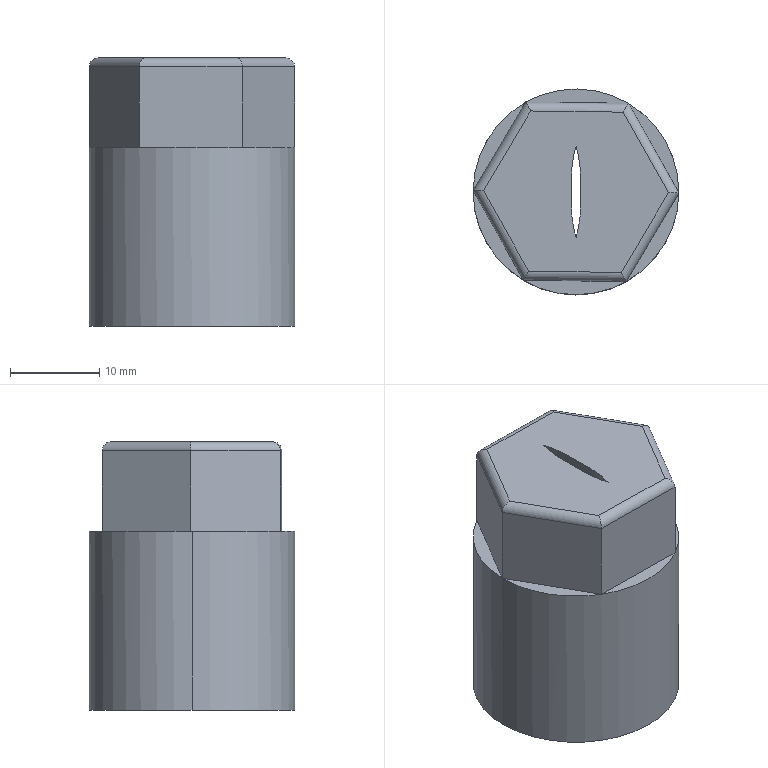Part | SolidWorks | features ICE 3, Extrusion 1, Fillet 1 | 1 solid | 35 faces | box 23 x 23 x 30 mm | volume 5402 mm3 | plane 21 | cylinder 14 | commonest cylinder face diameters 2 x6 20 x4 21 x2 23 x2
STEP:
#1=CARTESIAN_POINT('',(10.5,0.,18.));
#2=VERTEX_POINT('',#1);
#3=CARTESIAN_POINT('',(-10.5,0.,18.));
#4=VERTEX_POINT('',#3);
#5=CARTESIAN_POINT('',(0.,0.,18.));
#6=DIRECTION('',(0.,0.,-1.));
#7=DIRECTION('',(-1.,0.,0.));
#8=AXIS2_PLACEMENT_3D('',#5,#6,#7);
#9=CIRCLE('',#8,10.5);
#10=EDGE_CURVE('',#2,#4,#9,.T.);
#11=ORIENTED_EDGE('',*,*,#10,.F.);
#12=CARTESIAN_POINT('',(10.5,0.,0.));
#13=VERTEX_POINT('',#12);
#14=CARTESIAN_POINT('',(10.5,0.,18.));
#15=DIRECTION('',(0.,0.,-1.));
#16=VECTOR('',#15,1000.);
#17=LINE('',#14,#16);
#18=EDGE_CURVE('',#2,#13,#17,.T.);
#19=ORIENTED_EDGE('',*,*,#18,.T.);
#20=CARTESIAN_POINT('',(-10.5,0.,0.));
#21=VERTEX_POINT('',#20);
#22=CARTESIAN_POINT('',(0.,0.,0.));
#23=DIRECTION('',(0.,0.,-1.));
#24=DIRECTION('',(-1.,0.,0.));
#25=AXIS2_PLACEMENT_3D('',#22,#23,#24);
#26=CIRCLE('',#25,10.5);
#27=EDGE_CURVE('',#13,#21,#26,.T.);
#28=ORIENTED_EDGE('',*,*,#27,.T.);
#29=CARTESIAN_POINT('',(-10.5,0.,18.));
#30=DIRECTION('',(0.,0.,-1.));
#31=VECTOR('',#30,1000.);
#32=LINE('',#29,#31);
#33=EDGE_CURVE('',#4,#21,#32,.T.);
#34=ORIENTED_EDGE('',*,*,#33,.F.);
#35=EDGE_LOOP('',(#11,#19,#28,#34));
#36=FACE_OUTER_BOUND('',#35,.T.);
#37=CARTESIAN_POINT('',(0.,0.,18.));
#38=DIRECTION('',(0.,0.,-1.));
#39=DIRECTION('',(-1.,0.,0.));
#40=AXIS2_PLACEMENT_3D('',#37,#38,#39);
#41=CYLINDRICAL_SURFACE('',#40,10.5);
#42=ADVANCED_FACE('',(#36),#41,.F.);
#43=CARTESIAN_POINT('',(11.5,0.,20.));
#44=VERTEX_POINT('',#43);
#45=CARTESIAN_POINT('',(5.876,9.886,20.));
#46=VERTEX_POINT('',#45);
#47=CARTESIAN_POINT('',(0.,0.,20.));
#48=DIRECTION('',(0.,0.,1.));
#49=DIRECTION('',(1.,0.,0.));
#50=AXIS2_PLACEMENT_3D('',#47,#48,#49);
#51=CIRCLE('',#50,11.5);
#52=EDGE_CURVE('',#44,#46,#51,.T.);
#53=ORIENTED_EDGE('',*,*,#52,.F.);
#54=CARTESIAN_POINT('',(11.5,0.,0.));
#55=VERTEX_POINT('',#54);
#56=CARTESIAN_POINT('',(11.5,0.,30.));
#57=DIRECTION('',(0.,0.,-1.));
#58=VECTOR('',#57,1000.);
#59=LINE('',#56,#58);
#60=EDGE_CURVE('',#44,#55,#59,.T.);
#61=ORIENTED_EDGE('',*,*,#60,.T.);
#62=CARTESIAN_POINT('',(-11.5,0.,0.));
#63=VERTEX_POINT('',#62);
#64=CARTESIAN_POINT('',(0.,0.,0.));
#65=DIRECTION('',(0.,0.,1.));
#66=DIRECTION('',(1.,0.,0.));
#67=AXIS2_PLACEMENT_3D('',#64,#65,#66);
#68=CIRCLE('',#67,11.5);
#69=EDGE_CURVE('',#55,#63,#68,.T.);
#70=ORIENTED_EDGE('',*,*,#69,.T.);
#71=CARTESIAN_POINT('',(-11.5,0.,20.));
#72=VERTEX_POINT('',#71);
#73=CARTESIAN_POINT('',(-11.5,0.,30.));
#74=DIRECTION('',(0.,0.,-1.));
#75=VECTOR('',#74,1000.);
#76=LINE('',#73,#75);
#77=EDGE_CURVE('',#72,#63,#76,.T.);
#78=ORIENTED_EDGE('',*,*,#77,.F.);
#79=CARTESIAN_POINT('',(-11.499,0.1458,20.));
#80=VERTEX_POINT('',#79);
#81=CARTESIAN_POINT('',(0.,0.,20.));
#82=DIRECTION('',(0.,0.,1.));
#83=DIRECTION('',(1.,0.,0.));
#84=AXIS2_PLACEMENT_3D('',#81,#82,#83);
#85=CIRCLE('',#84,11.5);
#86=EDGE_CURVE('',#80,#72,#85,.T.);
#87=ORIENTED_EDGE('',*,*,#86,.F.);
#88=CARTESIAN_POINT('',(-5.623,10.031,20.));
#89=VERTEX_POINT('',#88);
#90=CARTESIAN_POINT('',(0.,0.,20.));
#91=DIRECTION('',(0.,0.,1.));
#92=DIRECTION('',(1.,0.,0.));
#93=AXIS2_PLACEMENT_3D('',#90,#91,#92);
#94=CIRCLE('',#93,11.5);
#95=EDGE_CURVE('',#89,#80,#94,.T.);
#96=ORIENTED_EDGE('',*,*,#95,.F.);
#97=CARTESIAN_POINT('',(0.,0.,20.));
#98=DIRECTION('',(0.,0.,1.));
#99=DIRECTION('',(1.,0.,0.));
#100=AXIS2_PLACEMENT_3D('',#97,#98,#99);
#101=CIRCLE('',#100,11.5);
#102=EDGE_CURVE('',#46,#89,#101,.T.);
#103=ORIENTED_EDGE('',*,*,#102,.F.);
#104=EDGE_LOOP('',(#53,#61,#70,#78,#87,#96,#103));
#105=FACE_OUTER_BOUND('',#104,.T.);
#106=CARTESIAN_POINT('',(0.,0.,30.));
#107=DIRECTION('',(0.,0.,-1.));
#108=DIRECTION('',(-1.,0.,0.));
#109=AXIS2_PLACEMENT_3D('',#106,#107,#108);
#110=CYLINDRICAL_SURFACE('',#109,11.5);
#111=ADVANCED_FACE('',(#105),#110,.T.);
#112=CARTESIAN_POINT('',(-0.2252,4.148,18.));
#113=VERTEX_POINT('',#112);
#114=CARTESIAN_POINT('',(-0.5,1.82,18.));
#115=VERTEX_POINT('',#114);
#116=CARTESIAN_POINT('',(9.5,1.82,18.));
#117=DIRECTION('',(0.,0.,1.));
#118=DIRECTION('',(-1.,0.,0.));
#119=AXIS2_PLACEMENT_3D('',#116,#117,#118);
#120=CIRCLE('',#119,10.);
#121=EDGE_CURVE('',#113,#115,#120,.T.);
#122=ORIENTED_EDGE('',*,*,#121,.F.);
#123=CARTESIAN_POINT('',(-0.2252,4.148,30.));
#124=VERTEX_POINT('',#123);
#125=CARTESIAN_POINT('',(-0.2252,4.148,0.));
#126=DIRECTION('',(0.,0.,1.));
#127=VECTOR('',#126,1000.);
#128=LINE('',#125,#127);
#129=EDGE_CURVE('',#113,#124,#128,.T.);
#130=ORIENTED_EDGE('',*,*,#129,.T.);
#131=CARTESIAN_POINT('',(-0.5,1.82,30.));
#132=VERTEX_POINT('',#131);
#133=CARTESIAN_POINT('',(9.5,1.82,30.));
#134=DIRECTION('',(0.,0.,1.));
#135=DIRECTION('',(-1.,0.,0.));
#136=AXIS2_PLACEMENT_3D('',#133,#134,#135);
#137=CIRCLE('',#136,10.);
#138=EDGE_CURVE('',#124,#132,#137,.T.);
#139=ORIENTED_EDGE('',*,*,#138,.T.);
#140=CARTESIAN_POINT('',(-0.5,1.82,0.));
#141=DIRECTION('',(0.,0.,1.));
#142=VECTOR('',#141,1000.);
#143=LINE('',#140,#142);
#144=EDGE_CURVE('',#115,#132,#143,.T.);
#145=ORIENTED_EDGE('',*,*,#144,.F.);
#146=EDGE_LOOP('',(#122,#130,#139,#145));
#147=FACE_OUTER_BOUND('',#146,.T.);
#148=CARTESIAN_POINT('',(9.5,1.82,0.));
#149=DIRECTION('',(0.,0.,1.));
#150=DIRECTION('',(1.,0.,0.));
#151=AXIS2_PLACEMENT_3D('',#148,#149,#150);
#152=CYLINDRICAL_SURFACE('',#151,10.);
#153=ADVANCED_FACE('',(#147),#152,.F.);
#154=CARTESIAN_POINT('',(0.,5.089,18.));
#155=VERTEX_POINT('',#154);
#156=CARTESIAN_POINT('',(-0.2252,4.148,18.));
#157=DIRECTION('',(-0.2328,-0.9725,0.));
#158=VECTOR('',#157,1000.);
#159=LINE('',#156,#158);
#160=EDGE_CURVE('',#155,#113,#159,.T.);
#161=ORIENTED_EDGE('',*,*,#160,.F.);
#162=CARTESIAN_POINT('',(0.,5.089,30.));
#163=VERTEX_POINT('',#162);
#164=CARTESIAN_POINT('',(0.,5.089,0.));
#165=DIRECTION('',(0.,0.,1.));
#166=VECTOR('',#165,1000.);
#167=LINE('',#164,#166);
#168=EDGE_CURVE('',#155,#163,#167,.T.);
#169=ORIENTED_EDGE('',*,*,#168,.T.);
#170=CARTESIAN_POINT('',(-0.2252,4.148,30.));
#171=DIRECTION('',(-0.2328,-0.9725,0.));
#172=VECTOR('',#171,1000.);
#173=LINE('',#170,#172);
#174=EDGE_CURVE('',#163,#124,#173,.T.);
#175=ORIENTED_EDGE('',*,*,#174,.T.);
#176=ORIENTED_EDGE('',*,*,#129,.F.);
#177=EDGE_LOOP('',(#161,#169,#175,#176));
#178=FACE_OUTER_BOUND('',#177,.T.);
#179=CARTESIAN_POINT('',(-0.2252,4.148,0.));
#180=DIRECTION('',(-0.9725,0.2328,0.));
#181=DIRECTION('',(-0.2328,-0.9725,0.));
#182=AXIS2_PLACEMENT_3D('',#179,#180,#181);
#183=PLANE('',#182);
#184=ADVANCED_FACE('',(#178),#183,.F.);
#185=CARTESIAN_POINT('',(0.2252,4.148,18.));
#186=VERTEX_POINT('',#185);
#187=CARTESIAN_POINT('',(0.,5.089,18.));
#188=DIRECTION('',(-0.2328,0.9725,0.));
#189=VECTOR('',#188,1000.);
#190=LINE('',#187,#189);
#191=EDGE_CURVE('',#186,#155,#190,.T.);
#192=ORIENTED_EDGE('',*,*,#191,.F.);
#193=CARTESIAN_POINT('',(0.2252,4.148,30.));
#194=VERTEX_POINT('',#193);
#195=CARTESIAN_POINT('',(0.2252,4.148,0.));
#196=DIRECTION('',(0.,0.,1.));
#197=VECTOR('',#196,1000.);
#198=LINE('',#195,#197);
#199=EDGE_CURVE('',#186,#194,#198,.T.);
#200=ORIENTED_EDGE('',*,*,#199,.T.);
#201=CARTESIAN_POINT('',(0.,5.089,30.));
#202=DIRECTION('',(-0.2328,0.9725,0.));
#203=VECTOR('',#202,1000.);
#204=LINE('',#201,#203);
#205=EDGE_CURVE('',#194,#163,#204,.T.);
#206=ORIENTED_EDGE('',*,*,#205,.T.);
#207=ORIENTED_EDGE('',*,*,#168,.F.);
#208=EDGE_LOOP('',(#192,#200,#206,#207));
#209=FACE_OUTER_BOUND('',#208,.T.);
#210=CARTESIAN_POINT('',(0.,5.089,0.));
#211=DIRECTION('',(0.9725,0.2328,0.));
#212=DIRECTION('',(-0.2328,0.9725,0.));
#213=AXIS2_PLACEMENT_3D('',#210,#211,#212);
#214=PLANE('',#213);
#215=ADVANCED_FACE('',(#209),#214,.F.);
#216=CARTESIAN_POINT('',(0.5,1.82,18.));
#217=VERTEX_POINT('',#216);
#218=CARTESIAN_POINT('',(-9.5,1.82,18.));
#219=DIRECTION('',(0.,0.,1.));
#220=DIRECTION('',(-1.,0.,0.));
#221=AXIS2_PLACEMENT_3D('',#218,#219,#220);
#222=CIRCLE('',#221,10.);
#223=EDGE_CURVE('',#217,#186,#222,.T.);
#224=ORIENTED_EDGE('',*,*,#223,.F.);
#225=CARTESIAN_POINT('',(0.5,1.82,30.));
#226=VERTEX_POINT('',#225);
#227=CARTESIAN_POINT('',(0.5,1.82,0.));
#228=DIRECTION('',(0.,0.,1.));
#229=VECTOR('',#228,1000.);
#230=LINE('',#227,#229);
#231=EDGE_CURVE('',#217,#226,#230,.T.);
#232=ORIENTED_EDGE('',*,*,#231,.T.);
#233=CARTESIAN_POINT('',(-9.5,1.82,30.));
#234=DIRECTION('',(0.,0.,1.));
#235=DIRECTION('',(1.,0.,0.));
#236=AXIS2_PLACEMENT_3D('',#233,#234,#235);
#237=CIRCLE('',#236,10.);
#238=EDGE_CURVE('',#226,#194,#237,.T.);
#239=ORIENTED_EDGE('',*,*,#238,.T.);
#240=ORIENTED_EDGE('',*,*,#199,.F.);
#241=EDGE_LOOP('',(#224,#232,#239,#240));
#242=FACE_OUTER_BOUND('',#241,.T.);
#243=CARTESIAN_POINT('',(-9.5,1.82,0.));
#244=DIRECTION('',(0.,0.,1.));
#245=DIRECTION('',(1.,0.,0.));
#246=AXIS2_PLACEMENT_3D('',#243,#244,#245);
#247=CYLINDRICAL_SURFACE('',#246,10.);
#248=ADVANCED_FACE('',(#242),#247,.F.);
#249=CARTESIAN_POINT('',(0.5,-1.82,18.));
#250=VERTEX_POINT('',#249);
#251=CARTESIAN_POINT('',(0.5,0.,18.));
#252=DIRECTION('',(0.,1.,0.));
#253=VECTOR('',#252,1000.);
#254=LINE('',#251,#253);
#255=EDGE_CURVE('',#250,#217,#254,.T.);
#256=ORIENTED_EDGE('',*,*,#255,.F.);
#257=CARTESIAN_POINT('',(0.5,-1.82,30.));
#258=VERTEX_POINT('',#257);
#259=CARTESIAN_POINT('',(0.5,-1.82,0.));
#260=DIRECTION('',(0.,0.,1.));
#261=VECTOR('',#260,1000.);
#262=LINE('',#259,#261);
#263=EDGE_CURVE('',#250,#258,#262,.T.);
#264=ORIENTED_EDGE('',*,*,#263,.T.);
#265=CARTESIAN_POINT('',(0.5,0.,30.));
#266=DIRECTION('',(0.,1.,0.));
#267=VECTOR('',#266,1000.);
#268=LINE('',#265,#267);
#269=EDGE_CURVE('',#258,#226,#268,.T.);
#270=ORIENTED_EDGE('',*,*,#269,.T.);
#271=ORIENTED_EDGE('',*,*,#231,.F.);
#272=EDGE_LOOP('',(#256,#264,#270,#271));
#273=FACE_OUTER_BOUND('',#272,.T.);
#274=CARTESIAN_POINT('',(0.5,0.,0.));
#275=DIRECTION('',(1.,0.,0.));
#276=DIRECTION('',(0.,0.,-1.));
#277=AXIS2_PLACEMENT_3D('',#274,#275,#276);
#278=PLANE('',#277);
#279=ADVANCED_FACE('',(#273),#278,.F.);
#280=CARTESIAN_POINT('',(0.2252,-4.148,18.));
#281=VERTEX_POINT('',#280);
#282=CARTESIAN_POINT('',(-9.5,-1.82,18.));
#283=DIRECTION('',(0.,0.,1.));
#284=DIRECTION('',(-1.,0.,0.));
#285=AXIS2_PLACEMENT_3D('',#282,#283,#284);
#286=CIRCLE('',#285,10.);
#287=EDGE_CURVE('',#281,#250,#286,.T.);
#288=ORIENTED_EDGE('',*,*,#287,.F.);
#289=CARTESIAN_POINT('',(0.2252,-4.148,30.));
#290=VERTEX_POINT('',#289);
#291=CARTESIAN_POINT('',(0.2252,-4.148,0.));
#292=DIRECTION('',(0.,0.,1.));
#293=VECTOR('',#292,1000.);
#294=LINE('',#291,#293);
#295=EDGE_CURVE('',#281,#290,#294,.T.);
#296=ORIENTED_EDGE('',*,*,#295,.T.);
#297=CARTESIAN_POINT('',(-9.5,-1.82,30.));
#298=DIRECTION('',(0.,0.,1.));
#299=DIRECTION('',(1.,0.,0.));
#300=AXIS2_PLACEMENT_3D('',#297,#298,#299);
#301=CIRCLE('',#300,10.);
#302=EDGE_CURVE('',#290,#258,#301,.T.);
#303=ORIENTED_EDGE('',*,*,#302,.T.);
#304=ORIENTED_EDGE('',*,*,#263,.F.);
#305=EDGE_LOOP('',(#288,#296,#303,#304));
#306=FACE_OUTER_BOUND('',#305,.T.);
#307=CARTESIAN_POINT('',(-9.5,-1.82,0.));
#308=DIRECTION('',(0.,0.,1.));
#309=DIRECTION('',(1.,0.,0.));
#310=AXIS2_PLACEMENT_3D('',#307,#308,#309);
#311=CYLINDRICAL_SURFACE('',#310,10.);
#312=ADVANCED_FACE('',(#306),#311,.F.);
#313=CARTESIAN_POINT('',(0.,-5.089,18.));
#314=VERTEX_POINT('',#313);
#315=CARTESIAN_POINT('',(0.,-5.089,18.));
#316=DIRECTION('',(0.2328,0.9725,0.));
#317=VECTOR('',#316,1000.);
#318=LINE('',#315,#317);
#319=EDGE_CURVE('',#314,#281,#318,.T.);
#320=ORIENTED_EDGE('',*,*,#319,.F.);
#321=CARTESIAN_POINT('',(0.,-5.089,30.));
#322=VERTEX_POINT('',#321);
#323=CARTESIAN_POINT('',(0.,-5.089,0.));
#324=DIRECTION('',(0.,0.,1.));
#325=VECTOR('',#324,1000.);
#326=LINE('',#323,#325);
#327=EDGE_CURVE('',#314,#322,#326,.T.);
#328=ORIENTED_EDGE('',*,*,#327,.T.);
#329=CARTESIAN_POINT('',(0.,-5.089,30.));
#330=DIRECTION('',(0.2328,0.9725,0.));
#331=VECTOR('',#330,1000.);
#332=LINE('',#329,#331);
#333=EDGE_CURVE('',#322,#290,#332,.T.);
#334=ORIENTED_EDGE('',*,*,#333,.T.);
#335=ORIENTED_EDGE('',*,*,#295,.F.);
#336=EDGE_LOOP('',(#320,#328,#334,#335));
#337=FACE_OUTER_BOUND('',#336,.T.);
#338=CARTESIAN_POINT('',(0.,-5.089,0.));
#339=DIRECTION('',(0.9725,-0.2328,0.));
#340=DIRECTION('',(0.2328,0.9725,0.));
#341=AXIS2_PLACEMENT_3D('',#338,#339,#340);
#342=PLANE('',#341);
#343=ADVANCED_FACE('',(#337),#342,.F.);
#344=CARTESIAN_POINT('',(-0.2252,-4.148,18.));
#345=VERTEX_POINT('',#344);
#346=CARTESIAN_POINT('',(-0.2252,-4.148,18.));
#347=DIRECTION('',(0.2328,-0.9725,0.));
#348=VECTOR('',#347,1000.);
#349=LINE('',#346,#348);
#350=EDGE_CURVE('',#345,#314,#349,.T.);
#351=ORIENTED_EDGE('',*,*,#350,.F.);
#352=CARTESIAN_POINT('',(-0.2252,-4.148,30.));
#353=VERTEX_POINT('',#352);
#354=CARTESIAN_POINT('',(-0.2252,-4.148,0.));
#355=DIRECTION('',(0.,0.,1.));
#356=VECTOR('',#355,1000.);
#357=LINE('',#354,#356);
#358=EDGE_CURVE('',#345,#353,#357,.T.);
#359=ORIENTED_EDGE('',*,*,#358,.T.);
#360=CARTESIAN_POINT('',(-0.2252,-4.148,30.));
#361=DIRECTION('',(0.2328,-0.9725,0.));
#362=VECTOR('',#361,1000.);
#363=LINE('',#360,#362);
#364=EDGE_CURVE('',#353,#322,#363,.T.);
#365=ORIENTED_EDGE('',*,*,#364,.T.);
#366=ORIENTED_EDGE('',*,*,#327,.F.);
#367=EDGE_LOOP('',(#351,#359,#365,#366));
#368=FACE_OUTER_BOUND('',#367,.T.);
#369=CARTESIAN_POINT('',(-0.2252,-4.148,0.));
#370=DIRECTION('',(-0.9725,-0.2328,0.));
#371=DIRECTION('',(0.2328,-0.9725,0.));
#372=AXIS2_PLACEMENT_3D('',#369,#370,#371);
#373=PLANE('',#372);
#374=ADVANCED_FACE('',(#368),#373,.F.);
#375=CARTESIAN_POINT('',(-0.5,-1.82,18.));
#376=VERTEX_POINT('',#375);
#377=CARTESIAN_POINT('',(9.5,-1.82,18.));
#378=DIRECTION('',(0.,0.,1.));
#379=DIRECTION('',(-1.,0.,0.));
#380=AXIS2_PLACEMENT_3D('',#377,#378,#379);
#381=CIRCLE('',#380,10.);
#382=EDGE_CURVE('',#376,#345,#381,.T.);
#383=ORIENTED_EDGE('',*,*,#382,.F.);
#384=CARTESIAN_POINT('',(-0.5,-1.82,30.));
#385=VERTEX_POINT('',#384);
#386=CARTESIAN_POINT('',(-0.5,-1.82,0.));
#387=DIRECTION('',(0.,0.,1.));
#388=VECTOR('',#387,1000.);
#389=LINE('',#386,#388);
#390=EDGE_CURVE('',#376,#385,#389,.T.);
#391=ORIENTED_EDGE('',*,*,#390,.T.);
#392=CARTESIAN_POINT('',(9.5,-1.82,30.));
#393=DIRECTION('',(0.,0.,1.));
#394=DIRECTION('',(1.,0.,0.));
#395=AXIS2_PLACEMENT_3D('',#392,#393,#394);
#396=CIRCLE('',#395,10.);
#397=EDGE_CURVE('',#385,#353,#396,.T.);
#398=ORIENTED_EDGE('',*,*,#397,.T.);
#399=ORIENTED_EDGE('',*,*,#358,.F.);
#400=EDGE_LOOP('',(#383,#391,#398,#399));
#401=FACE_OUTER_BOUND('',#400,.T.);
#402=CARTESIAN_POINT('',(9.5,-1.82,0.));
#403=DIRECTION('',(0.,0.,1.));
#404=DIRECTION('',(1.,0.,0.));
#405=AXIS2_PLACEMENT_3D('',#402,#403,#404);
#406=CYLINDRICAL_SURFACE('',#405,10.);
#407=ADVANCED_FACE('',(#401),#406,.F.);
#408=CARTESIAN_POINT('',(-0.5,0.,18.));
#409=DIRECTION('',(0.,-1.,0.));
#410=VECTOR('',#409,1000.);
#411=LINE('',#408,#410);
#412=EDGE_CURVE('',#115,#376,#411,.T.);
#413=ORIENTED_EDGE('',*,*,#412,.F.);
#414=ORIENTED_EDGE('',*,*,#144,.T.);
#415=CARTESIAN_POINT('',(-0.5,0.,30.));
#416=DIRECTION('',(0.,-1.,0.));
#417=VECTOR('',#416,1000.);
#418=LINE('',#415,#417);
#419=EDGE_CURVE('',#132,#385,#418,.T.);
#420=ORIENTED_EDGE('',*,*,#419,.T.);
#421=ORIENTED_EDGE('',*,*,#390,.F.);
#422=EDGE_LOOP('',(#413,#414,#420,#421));
#423=FACE_OUTER_BOUND('',#422,.T.);
#424=CARTESIAN_POINT('',(-0.5,0.,0.));
#425=DIRECTION('',(-1.,0.,0.));
#426=DIRECTION('',(0.,-1.,0.));
#427=AXIS2_PLACEMENT_3D('',#424,#425,#426);
#428=PLANE('',#427);
#429=ADVANCED_FACE('',(#423),#428,.F.);
#430=ORIENTED_EDGE('',*,*,#60,.F.);
#431=CARTESIAN_POINT('',(11.499,-0.1458,20.));
#432=VERTEX_POINT('',#431);
#433=CARTESIAN_POINT('',(0.,0.,20.));
#434=DIRECTION('',(0.,0.,1.));
#435=DIRECTION('',(1.,0.,0.));
#436=AXIS2_PLACEMENT_3D('',#433,#434,#435);
#437=CIRCLE('',#436,11.5);
#438=EDGE_CURVE('',#432,#44,#437,.T.);
#439=ORIENTED_EDGE('',*,*,#438,.F.);
#440=CARTESIAN_POINT('',(5.623,-10.031,20.));
#441=VERTEX_POINT('',#440);
#442=CARTESIAN_POINT('',(0.,0.,20.));
#443=DIRECTION('',(0.,0.,1.));
#444=DIRECTION('',(1.,0.,0.));
#445=AXIS2_PLACEMENT_3D('',#442,#443,#444);
#446=CIRCLE('',#445,11.5);
#447=EDGE_CURVE('',#441,#432,#446,.T.);
#448=ORIENTED_EDGE('',*,*,#447,.F.);
#449=CARTESIAN_POINT('',(-5.876,-9.886,20.));
#450=VERTEX_POINT('',#449);
#451=CARTESIAN_POINT('',(0.,0.,20.));
#452=DIRECTION('',(0.,0.,1.));
#453=DIRECTION('',(1.,0.,0.));
#454=AXIS2_PLACEMENT_3D('',#451,#452,#453);
#455=CIRCLE('',#454,11.5);
#456=EDGE_CURVE('',#450,#441,#455,.T.);
#457=ORIENTED_EDGE('',*,*,#456,.F.);
#458=CARTESIAN_POINT('',(0.,0.,20.));
#459=DIRECTION('',(0.,0.,1.));
#460=DIRECTION('',(1.,0.,0.));
#461=AXIS2_PLACEMENT_3D('',#458,#459,#460);
#462=CIRCLE('',#461,11.5);
#463=EDGE_CURVE('',#72,#450,#462,.T.);
#464=ORIENTED_EDGE('',*,*,#463,.F.);
#465=ORIENTED_EDGE('',*,*,#77,.T.);
#466=CARTESIAN_POINT('',(0.,0.,0.));
#467=DIRECTION('',(0.,0.,1.));
#468=DIRECTION('',(1.,0.,0.));
#469=AXIS2_PLACEMENT_3D('',#466,#467,#468);
#470=CIRCLE('',#469,11.5);
#471=EDGE_CURVE('',#63,#55,#470,.T.);
#472=ORIENTED_EDGE('',*,*,#471,.T.);
#473=EDGE_LOOP('',(#430,#439,#448,#457,#464,#465,#472));
#474=FACE_OUTER_BOUND('',#473,.T.);
#475=CARTESIAN_POINT('',(0.,0.,30.));
#476=DIRECTION('',(0.,0.,-1.));
#477=DIRECTION('',(-1.,0.,0.));
#478=AXIS2_PLACEMENT_3D('',#475,#476,#477);
#479=CYLINDRICAL_SURFACE('',#478,11.5);
#480=ADVANCED_FACE('',(#474),#479,.T.);
#481=CARTESIAN_POINT('',(0.,0.,0.));
#482=DIRECTION('',(0.,0.,-1.));
#483=DIRECTION('',(-1.,0.,0.));
#484=AXIS2_PLACEMENT_3D('',#481,#482,#483);
#485=CIRCLE('',#484,10.5);
#486=EDGE_CURVE('',#21,#13,#485,.T.);
#487=ORIENTED_EDGE('',*,*,#486,.F.);
#488=ORIENTED_EDGE('',*,*,#27,.F.);
#489=EDGE_LOOP('',(#487,#488));
#490=FACE_BOUND('',#489,.T.);
#491=ORIENTED_EDGE('',*,*,#471,.F.);
#492=ORIENTED_EDGE('',*,*,#69,.F.);
#493=EDGE_LOOP('',(#491,#492));
#494=FACE_OUTER_BOUND('',#493,.T.);
#495=CARTESIAN_POINT('',(0.,0.,0.));
#496=DIRECTION('',(0.,0.,1.));
#497=DIRECTION('',(1.,0.,0.));
#498=AXIS2_PLACEMENT_3D('',#495,#496,#497);
#499=PLANE('',#498);
#500=ADVANCED_FACE('',(#490,#494),#499,.F.);
#501=ORIENTED_EDGE('',*,*,#102,.T.);
#502=CARTESIAN_POINT('',(5.876,9.886,20.));
#503=DIRECTION('',(-0.9999,0.01268,0.));
#504=VECTOR('',#503,1000.);
#505=LINE('',#502,#504);
#506=EDGE_CURVE('',#46,#89,#505,.T.);
#507=ORIENTED_EDGE('',*,*,#506,.F.);
#508=EDGE_LOOP('',(#501,#507));
#509=FACE_OUTER_BOUND('',#508,.T.);
#510=CARTESIAN_POINT('',(0.,0.,20.));
#511=DIRECTION('',(0.,0.,1.));
#512=DIRECTION('',(1.,0.,0.));
#513=AXIS2_PLACEMENT_3D('',#510,#511,#512);
#514=PLANE('',#513);
#515=ADVANCED_FACE('',(#509),#514,.T.);
#516=ORIENTED_EDGE('',*,*,#95,.T.);
#517=CARTESIAN_POINT('',(-5.623,10.031,20.));
#518=DIRECTION('',(-0.5109,-0.8596,0.));
#519=VECTOR('',#518,1000.);
#520=LINE('',#517,#519);
#521=EDGE_CURVE('',#89,#80,#520,.T.);
#522=ORIENTED_EDGE('',*,*,#521,.F.);
#523=EDGE_LOOP('',(#516,#522));
#524=FACE_OUTER_BOUND('',#523,.T.);
#525=CARTESIAN_POINT('',(0.,0.,20.));
#526=DIRECTION('',(0.,0.,1.));
#527=DIRECTION('',(1.,0.,0.));
#528=AXIS2_PLACEMENT_3D('',#525,#526,#527);
#529=PLANE('',#528);
#530=ADVANCED_FACE('',(#524),#529,.T.);
#531=ORIENTED_EDGE('',*,*,#86,.T.);
#532=ORIENTED_EDGE('',*,*,#463,.T.);
#533=CARTESIAN_POINT('',(-11.499,0.1458,20.));
#534=DIRECTION('',(0.489,-0.8723,0.));
#535=VECTOR('',#534,1000.);
#536=LINE('',#533,#535);
#537=EDGE_CURVE('',#80,#450,#536,.T.);
#538=ORIENTED_EDGE('',*,*,#537,.F.);
#539=EDGE_LOOP('',(#531,#532,#538));
#540=FACE_OUTER_BOUND('',#539,.T.);
#541=CARTESIAN_POINT('',(0.,0.,20.));
#542=DIRECTION('',(0.,0.,1.));
#543=DIRECTION('',(1.,0.,0.));
#544=AXIS2_PLACEMENT_3D('',#541,#542,#543);
#545=PLANE('',#544);
#546=ADVANCED_FACE('',(#540),#545,.T.);
#547=ORIENTED_EDGE('',*,*,#456,.T.);
#548=CARTESIAN_POINT('',(-5.876,-9.886,20.));
#549=DIRECTION('',(0.9999,-0.01268,0.));
#550=VECTOR('',#549,1000.);
#551=LINE('',#548,#550);
#552=EDGE_CURVE('',#450,#441,#551,.T.);
#553=ORIENTED_EDGE('',*,*,#552,.F.);
#554=EDGE_LOOP('',(#547,#553));
#555=FACE_OUTER_BOUND('',#554,.T.);
#556=CARTESIAN_POINT('',(0.,0.,20.));
#557=DIRECTION('',(0.,0.,1.));
#558=DIRECTION('',(1.,0.,0.));
#559=AXIS2_PLACEMENT_3D('',#556,#557,#558);
#560=PLANE('',#559);
#561=ADVANCED_FACE('',(#555),#560,.T.);
#562=ORIENTED_EDGE('',*,*,#447,.T.);
#563=CARTESIAN_POINT('',(5.623,-10.031,20.));
#564=DIRECTION('',(0.5109,0.8596,0.));
#565=VECTOR('',#564,1000.);
#566=LINE('',#563,#565);
#567=EDGE_CURVE('',#441,#432,#566,.T.);
#568=ORIENTED_EDGE('',*,*,#567,.F.);
#569=EDGE_LOOP('',(#562,#568));
#570=FACE_OUTER_BOUND('',#569,.T.);
#571=CARTESIAN_POINT('',(0.,0.,20.));
#572=DIRECTION('',(0.,0.,1.));
#573=DIRECTION('',(1.,0.,0.));
#574=AXIS2_PLACEMENT_3D('',#571,#572,#573);
#575=PLANE('',#574);
#576=ADVANCED_FACE('',(#570),#575,.T.);
#577=ORIENTED_EDGE('',*,*,#438,.T.);
#578=ORIENTED_EDGE('',*,*,#52,.T.);
#579=CARTESIAN_POINT('',(11.499,-0.1458,20.));
#580=DIRECTION('',(-0.489,0.8723,0.));
#581=VECTOR('',#580,1000.);
#582=LINE('',#579,#581);
#583=EDGE_CURVE('',#432,#46,#582,.T.);
#584=ORIENTED_EDGE('',*,*,#583,.F.);
#585=EDGE_LOOP('',(#577,#578,#584));
#586=FACE_OUTER_BOUND('',#585,.T.);
#587=CARTESIAN_POINT('',(0.,0.,20.));
#588=DIRECTION('',(0.,0.,1.));
#589=DIRECTION('',(1.,0.,0.));
#590=AXIS2_PLACEMENT_3D('',#587,#588,#589);
#591=PLANE('',#590);
#592=ADVANCED_FACE('',(#586),#591,.T.);
#593=CARTESIAN_POINT('',(5.876,9.886,29.));
#594=VERTEX_POINT('',#593);
#595=CARTESIAN_POINT('',(5.876,9.886,20.));
#596=DIRECTION('',(0.,0.,1.));
#597=VECTOR('',#596,1000.);
#598=LINE('',#595,#597);
#599=EDGE_CURVE('',#46,#594,#598,.T.);
#600=ORIENTED_EDGE('',*,*,#599,.T.);
#601=CARTESIAN_POINT('',(11.499,-0.1458,29.));
#602=VERTEX_POINT('',#601);
#603=CARTESIAN_POINT('',(11.499,-0.1458,29.));
#604=DIRECTION('',(0.489,-0.8723,0.));
#605=VECTOR('',#604,1000.);
#606=LINE('',#603,#605);
#607=EDGE_CURVE('',#594,#602,#606,.T.);
#608=ORIENTED_EDGE('',*,*,#607,.T.);
#609=CARTESIAN_POINT('',(11.499,-0.1458,20.));
#610=DIRECTION('',(0.,0.,1.));
#611=VECTOR('',#610,1000.);
#612=LINE('',#609,#611);
#613=EDGE_CURVE('',#432,#602,#612,.T.);
#614=ORIENTED_EDGE('',*,*,#613,.F.);
#615=ORIENTED_EDGE('',*,*,#583,.T.);
#616=EDGE_LOOP('',(#600,#608,#614,#615));
#617=FACE_OUTER_BOUND('',#616,.T.);
#618=CARTESIAN_POINT('',(11.499,-0.1458,20.));
#619=DIRECTION('',(0.8723,0.489,0.));
#620=DIRECTION('',(-0.489,0.8723,0.));
#621=AXIS2_PLACEMENT_3D('',#618,#619,#620);
#622=PLANE('',#621);
#623=ADVANCED_FACE('',(#617),#622,.T.);
#624=ORIENTED_EDGE('',*,*,#613,.T.);
#625=CARTESIAN_POINT('',(5.623,-10.031,29.));
#626=VERTEX_POINT('',#625);
#627=CARTESIAN_POINT('',(5.623,-10.031,29.));
#628=DIRECTION('',(-0.5109,-0.8596,0.));
#629=VECTOR('',#628,1000.);
#630=LINE('',#627,#629);
#631=EDGE_CURVE('',#602,#626,#630,.T.);
#632=ORIENTED_EDGE('',*,*,#631,.T.);
#633=CARTESIAN_POINT('',(5.623,-10.031,20.));
#634=DIRECTION('',(0.,0.,1.));
#635=VECTOR('',#634,1000.);
#636=LINE('',#633,#635);
#637=EDGE_CURVE('',#441,#626,#636,.T.);
#638=ORIENTED_EDGE('',*,*,#637,.F.);
#639=ORIENTED_EDGE('',*,*,#567,.T.);
#640=EDGE_LOOP('',(#624,#632,#638,#639));
#641=FACE_OUTER_BOUND('',#640,.T.);
#642=CARTESIAN_POINT('',(5.623,-10.031,20.));
#643=DIRECTION('',(0.8596,-0.5109,0.));
#644=DIRECTION('',(0.5109,0.8596,0.));
#645=AXIS2_PLACEMENT_3D('',#642,#643,#644);
#646=PLANE('',#645);
#647=ADVANCED_FACE('',(#641),#646,.T.);
#648=ORIENTED_EDGE('',*,*,#637,.T.);
#649=CARTESIAN_POINT('',(-5.876,-9.886,29.));
#650=VERTEX_POINT('',#649);
#651=CARTESIAN_POINT('',(-5.876,-9.886,29.));
#652=DIRECTION('',(-0.9999,0.01268,0.));
#653=VECTOR('',#652,1000.);
#654=LINE('',#651,#653);
#655=EDGE_CURVE('',#626,#650,#654,.T.);
#656=ORIENTED_EDGE('',*,*,#655,.T.);
#657=CARTESIAN_POINT('',(-5.876,-9.886,20.));
#658=DIRECTION('',(0.,0.,1.));
#659=VECTOR('',#658,1000.);
#660=LINE('',#657,#659);
#661=EDGE_CURVE('',#450,#650,#660,.T.);
#662=ORIENTED_EDGE('',*,*,#661,.F.);
#663=ORIENTED_EDGE('',*,*,#552,.T.);
#664=EDGE_LOOP('',(#648,#656,#662,#663));
#665=FACE_OUTER_BOUND('',#664,.T.);
#666=CARTESIAN_POINT('',(-5.876,-9.886,20.));
#667=DIRECTION('',(-0.01268,-0.9999,0.));
#668=DIRECTION('',(0.9999,-0.01268,0.));
#669=AXIS2_PLACEMENT_3D('',#666,#667,#668);
#670=PLANE('',#669);
#671=ADVANCED_FACE('',(#665),#670,.T.);
#672=ORIENTED_EDGE('',*,*,#661,.T.);
#673=CARTESIAN_POINT('',(-11.499,0.1458,29.));
#674=VERTEX_POINT('',#673);
#675=CARTESIAN_POINT('',(-11.499,0.1458,29.));
#676=DIRECTION('',(-0.489,0.8723,0.));
#677=VECTOR('',#676,1000.);
#678=LINE('',#675,#677);
#679=EDGE_CURVE('',#650,#674,#678,.T.);
#680=ORIENTED_EDGE('',*,*,#679,.T.);
#681=CARTESIAN_POINT('',(-11.499,0.1458,20.));
#682=DIRECTION('',(0.,0.,1.));
#683=VECTOR('',#682,1000.);
#684=LINE('',#681,#683);
#685=EDGE_CURVE('',#80,#674,#684,.T.);
#686=ORIENTED_EDGE('',*,*,#685,.F.);
#687=ORIENTED_EDGE('',*,*,#537,.T.);
#688=EDGE_LOOP('',(#672,#680,#686,#687));
#689=FACE_OUTER_BOUND('',#688,.T.);
#690=CARTESIAN_POINT('',(-11.499,0.1458,20.));
#691=DIRECTION('',(-0.8723,-0.489,0.));
#692=DIRECTION('',(0.489,-0.8723,0.));
#693=AXIS2_PLACEMENT_3D('',#690,#691,#692);
#694=PLANE('',#693);
#695=ADVANCED_FACE('',(#689),#694,.T.);
#696=ORIENTED_EDGE('',*,*,#685,.T.);
#697=CARTESIAN_POINT('',(-5.623,10.031,29.));
#698=VERTEX_POINT('',#697);
#699=CARTESIAN_POINT('',(-5.623,10.031,29.));
#700=DIRECTION('',(0.5109,0.8596,0.));
#701=VECTOR('',#700,1000.);
#702=LINE('',#699,#701);
#703=EDGE_CURVE('',#674,#698,#702,.T.);
#704=ORIENTED_EDGE('',*,*,#703,.T.);
#705=CARTESIAN_POINT('',(-5.623,10.031,20.));
#706=DIRECTION('',(0.,0.,1.));
#707=VECTOR('',#706,1000.);
#708=LINE('',#705,#707);
#709=EDGE_CURVE('',#89,#698,#708,.T.);
#710=ORIENTED_EDGE('',*,*,#709,.F.);
#711=ORIENTED_EDGE('',*,*,#521,.T.);
#712=EDGE_LOOP('',(#696,#704,#710,#711));
#713=FACE_OUTER_BOUND('',#712,.T.);
#714=CARTESIAN_POINT('',(-5.623,10.031,20.));
#715=DIRECTION('',(-0.8596,0.5109,0.));
#716=DIRECTION('',(-0.5109,-0.8596,0.));
#717=AXIS2_PLACEMENT_3D('',#714,#715,#716);
#718=PLANE('',#717);
#719=ADVANCED_FACE('',(#713),#718,.T.);
#720=ORIENTED_EDGE('',*,*,#709,.T.);
#721=CARTESIAN_POINT('',(5.876,9.886,29.));
#722=DIRECTION('',(0.9999,-0.01268,0.));
#723=VECTOR('',#722,1000.);
#724=LINE('',#721,#723);
#725=EDGE_CURVE('',#698,#594,#724,.T.);
#726=ORIENTED_EDGE('',*,*,#725,.T.);
#727=ORIENTED_EDGE('',*,*,#599,.F.);
#728=ORIENTED_EDGE('',*,*,#506,.T.);
#729=EDGE_LOOP('',(#720,#726,#727,#728));
#730=FACE_OUTER_BOUND('',#729,.T.);
#731=CARTESIAN_POINT('',(5.876,9.886,20.));
#732=DIRECTION('',(0.01268,0.9999,0.));
#733=DIRECTION('',(-0.9999,0.01268,0.));
#734=AXIS2_PLACEMENT_3D('',#731,#732,#733);
#735=PLANE('',#734);
#736=ADVANCED_FACE('',(#730),#735,.T.);
#737=ORIENTED_EDGE('',*,*,#138,.F.);
#738=ORIENTED_EDGE('',*,*,#174,.F.);
#739=ORIENTED_EDGE('',*,*,#205,.F.);
#740=ORIENTED_EDGE('',*,*,#238,.F.);
#741=ORIENTED_EDGE('',*,*,#269,.F.);
#742=ORIENTED_EDGE('',*,*,#302,.F.);
#743=ORIENTED_EDGE('',*,*,#333,.F.);
#744=ORIENTED_EDGE('',*,*,#364,.F.);
#745=ORIENTED_EDGE('',*,*,#397,.F.);
#746=ORIENTED_EDGE('',*,*,#419,.F.);
#747=EDGE_LOOP('',(#737,#738,#739,#740,#741,#742,#743,#744,#745,#746));
#748=FACE_BOUND('',#747,.T.);
#749=CARTESIAN_POINT('',(-5.059,9.024,30.));
#750=VERTEX_POINT('',#749);
#751=CARTESIAN_POINT('',(-10.344,0.1311,30.));
#752=VERTEX_POINT('',#751);
#753=CARTESIAN_POINT('',(-7.702,4.578,30.));
#754=DIRECTION('',(-0.5109,-0.8596,0.));
#755=VECTOR('',#754,1000.);
#756=LINE('',#753,#755);
#757=EDGE_CURVE('',#750,#752,#756,.T.);
#758=ORIENTED_EDGE('',*,*,#757,.T.);
#759=CARTESIAN_POINT('',(-5.286,-8.893,30.));
#760=VERTEX_POINT('',#759);
#761=CARTESIAN_POINT('',(-7.815,-4.381,30.));
#762=DIRECTION('',(0.489,-0.8723,0.));
#763=VECTOR('',#762,1000.);
#764=LINE('',#761,#763);
#765=EDGE_CURVE('',#752,#760,#764,.T.);
#766=ORIENTED_EDGE('',*,*,#765,.T.);
#767=CARTESIAN_POINT('',(5.059,-9.024,30.));
#768=VERTEX_POINT('',#767);
#769=CARTESIAN_POINT('',(-0.1136,-8.959,30.));
#770=DIRECTION('',(0.9999,-0.01268,0.));
#771=VECTOR('',#770,1000.);
#772=LINE('',#769,#771);
#773=EDGE_CURVE('',#760,#768,#772,.T.);
#774=ORIENTED_EDGE('',*,*,#773,.T.);
#775=CARTESIAN_POINT('',(10.344,-0.1311,30.));
#776=VERTEX_POINT('',#775);
#777=CARTESIAN_POINT('',(7.702,-4.578,30.));
#778=DIRECTION('',(0.5109,0.8596,0.));
#779=VECTOR('',#778,1000.);
#780=LINE('',#777,#779);
#781=EDGE_CURVE('',#768,#776,#780,.T.);
#782=ORIENTED_EDGE('',*,*,#781,.T.);
#783=CARTESIAN_POINT('',(5.286,8.893,30.));
#784=VERTEX_POINT('',#783);
#785=CARTESIAN_POINT('',(7.815,4.381,30.));
#786=DIRECTION('',(-0.489,0.8723,0.));
#787=VECTOR('',#786,1000.);
#788=LINE('',#785,#787);
#789=EDGE_CURVE('',#776,#784,#788,.T.);
#790=ORIENTED_EDGE('',*,*,#789,.T.);
#791=CARTESIAN_POINT('',(0.1136,8.959,30.));
#792=DIRECTION('',(-0.9999,0.01268,0.));
#793=VECTOR('',#792,1000.);
#794=LINE('',#791,#793);
#795=EDGE_CURVE('',#784,#750,#794,.T.);
#796=ORIENTED_EDGE('',*,*,#795,.T.);
#797=EDGE_LOOP('',(#758,#766,#774,#782,#790,#796));
#798=FACE_OUTER_BOUND('',#797,.T.);
#799=CARTESIAN_POINT('',(0.,0.,30.));
#800=DIRECTION('',(0.,0.,1.));
#801=DIRECTION('',(1.,0.,0.));
#802=AXIS2_PLACEMENT_3D('',#799,#800,#801);
#803=PLANE('',#802);
#804=ADVANCED_FACE('',(#748,#798),#803,.T.);
#805=CARTESIAN_POINT('',(11.499,-0.1458,29.));
#806=CARTESIAN_POINT('',(11.499,-0.1458,29.586));
#807=CARTESIAN_POINT('',(11.021,-0.1397,30.));
#808=CARTESIAN_POINT('',(10.344,-0.1311,30.));
#809=(BOUNDED_CURVE()B_SPLINE_CURVE(3,(#805,#806,#807,#808),.UNSPECIFIED.,.F.,.F.)B_SPLINE_CURVE_WITH_KNOTS((4,4),(3.142,4.712),.UNSPECIFIED.)CURVE()GEOMETRIC_REPRESENTATION_ITEM()RATIONAL_B_SPLINE_CURVE((1.,0.8047,0.8047,1.))REPRESENTATION_ITEM(''));
#810=EDGE_CURVE('',#602,#776,#809,.T.);
#811=ORIENTED_EDGE('',*,*,#810,.F.);
#812=ORIENTED_EDGE('',*,*,#607,.F.);
#813=CARTESIAN_POINT('',(5.286,8.893,30.));
#814=CARTESIAN_POINT('',(5.631,9.474,30.));
#815=CARTESIAN_POINT('',(5.876,9.886,29.586));
#816=CARTESIAN_POINT('',(5.876,9.886,29.));
#817=(BOUNDED_CURVE()B_SPLINE_CURVE(3,(#813,#814,#815,#816),.UNSPECIFIED.,.F.,.F.)B_SPLINE_CURVE_WITH_KNOTS((4,4),(1.571,3.142),.UNSPECIFIED.)CURVE()GEOMETRIC_REPRESENTATION_ITEM()RATIONAL_B_SPLINE_CURVE((1.,0.8047,0.8047,1.))REPRESENTATION_ITEM(''));
#818=EDGE_CURVE('',#784,#594,#817,.T.);
#819=ORIENTED_EDGE('',*,*,#818,.F.);
#820=ORIENTED_EDGE('',*,*,#789,.F.);
#821=EDGE_LOOP('',(#811,#812,#819,#820));
#822=FACE_OUTER_BOUND('',#821,.T.);
#823=CARTESIAN_POINT('',(7.815,4.381,29.));
#824=DIRECTION('',(-0.489,0.8723,0.));
#825=DIRECTION('',(-0.8723,-0.489,0.));
#826=AXIS2_PLACEMENT_3D('',#823,#824,#825);
#827=CYLINDRICAL_SURFACE('',#826,1.);
#828=ADVANCED_FACE('',(#822),#827,.T.);
#829=ORIENTED_EDGE('',*,*,#818,.T.);
#830=ORIENTED_EDGE('',*,*,#725,.F.);
#831=CARTESIAN_POINT('',(-5.059,9.024,30.));
#832=CARTESIAN_POINT('',(-5.389,9.614,30.));
#833=CARTESIAN_POINT('',(-5.623,10.031,29.586));
#834=CARTESIAN_POINT('',(-5.623,10.031,29.));
#835=(BOUNDED_CURVE()B_SPLINE_CURVE(3,(#831,#832,#833,#834),.UNSPECIFIED.,.F.,.F.)B_SPLINE_CURVE_WITH_KNOTS((4,4),(1.571,3.142),.UNSPECIFIED.)CURVE()GEOMETRIC_REPRESENTATION_ITEM()RATIONAL_B_SPLINE_CURVE((1.,0.8047,0.8047,1.))REPRESENTATION_ITEM(''));
#836=EDGE_CURVE('',#750,#698,#835,.T.);
#837=ORIENTED_EDGE('',*,*,#836,.F.);
#838=ORIENTED_EDGE('',*,*,#795,.F.);
#839=EDGE_LOOP('',(#829,#830,#837,#838));
#840=FACE_OUTER_BOUND('',#839,.T.);
#841=CARTESIAN_POINT('',(0.1136,8.959,29.));
#842=DIRECTION('',(-0.9999,0.01268,0.));
#843=DIRECTION('',(-0.01268,-0.9999,0.));
#844=AXIS2_PLACEMENT_3D('',#841,#842,#843);
#845=CYLINDRICAL_SURFACE('',#844,1.);
#846=ADVANCED_FACE('',(#840),#845,.T.);
#847=ORIENTED_EDGE('',*,*,#810,.T.);
#848=ORIENTED_EDGE('',*,*,#781,.F.);
#849=CARTESIAN_POINT('',(5.623,-10.031,29.));
#850=CARTESIAN_POINT('',(5.623,-10.031,29.586));
#851=CARTESIAN_POINT('',(5.389,-9.614,30.));
#852=CARTESIAN_POINT('',(5.059,-9.024,30.));
#853=(BOUNDED_CURVE()B_SPLINE_CURVE(3,(#849,#850,#851,#852),.UNSPECIFIED.,.F.,.F.)B_SPLINE_CURVE_WITH_KNOTS((4,4),(3.142,4.712),.UNSPECIFIED.)CURVE()GEOMETRIC_REPRESENTATION_ITEM()RATIONAL_B_SPLINE_CURVE((1.,0.8047,0.8047,1.))REPRESENTATION_ITEM(''));
#854=EDGE_CURVE('',#626,#768,#853,.T.);
#855=ORIENTED_EDGE('',*,*,#854,.F.);
#856=ORIENTED_EDGE('',*,*,#631,.F.);
#857=EDGE_LOOP('',(#847,#848,#855,#856));
#858=FACE_OUTER_BOUND('',#857,.T.);
#859=CARTESIAN_POINT('',(7.702,-4.578,29.));
#860=DIRECTION('',(0.5109,0.8596,0.));
#861=DIRECTION('',(-0.8596,0.5109,0.));
#862=AXIS2_PLACEMENT_3D('',#859,#860,#861);
#863=CYLINDRICAL_SURFACE('',#862,1.);
#864=ADVANCED_FACE('',(#858),#863,.T.);
#865=ORIENTED_EDGE('',*,*,#836,.T.);
#866=ORIENTED_EDGE('',*,*,#703,.F.);
#867=CARTESIAN_POINT('',(-10.344,0.1311,30.));
#868=CARTESIAN_POINT('',(-11.021,0.1397,30.));
#869=CARTESIAN_POINT('',(-11.499,0.1458,29.586));
#870=CARTESIAN_POINT('',(-11.499,0.1458,29.));
#871=(BOUNDED_CURVE()B_SPLINE_CURVE(3,(#867,#868,#869,#870),.UNSPECIFIED.,.F.,.F.)B_SPLINE_CURVE_WITH_KNOTS((4,4),(4.712,6.283),.UNSPECIFIED.)CURVE()GEOMETRIC_REPRESENTATION_ITEM()RATIONAL_B_SPLINE_CURVE((1.,0.8047,0.8047,1.))REPRESENTATION_ITEM(''));
#872=EDGE_CURVE('',#752,#674,#871,.T.);
#873=ORIENTED_EDGE('',*,*,#872,.F.);
#874=ORIENTED_EDGE('',*,*,#757,.F.);
#875=EDGE_LOOP('',(#865,#866,#873,#874));
#876=FACE_OUTER_BOUND('',#875,.T.);
#877=CARTESIAN_POINT('',(-7.702,4.578,29.));
#878=DIRECTION('',(-0.5109,-0.8596,0.));
#879=DIRECTION('',(0.8596,-0.5109,0.));
#880=AXIS2_PLACEMENT_3D('',#877,#878,#879);
#881=CYLINDRICAL_SURFACE('',#880,1.);
#882=ADVANCED_FACE('',(#876),#881,.T.);
#883=ORIENTED_EDGE('',*,*,#854,.T.);
#884=ORIENTED_EDGE('',*,*,#773,.F.);
#885=CARTESIAN_POINT('',(-5.876,-9.886,29.));
#886=CARTESIAN_POINT('',(-5.876,-9.886,29.586));
#887=CARTESIAN_POINT('',(-5.631,-9.474,30.));
#888=CARTESIAN_POINT('',(-5.286,-8.893,30.));
#889=(BOUNDED_CURVE()B_SPLINE_CURVE(3,(#885,#886,#887,#888),.UNSPECIFIED.,.F.,.F.)B_SPLINE_CURVE_WITH_KNOTS((4,4),(3.142,4.712),.UNSPECIFIED.)CURVE()GEOMETRIC_REPRESENTATION_ITEM()RATIONAL_B_SPLINE_CURVE((1.,0.8047,0.8047,1.))REPRESENTATION_ITEM(''));
#890=EDGE_CURVE('',#650,#760,#889,.T.);
#891=ORIENTED_EDGE('',*,*,#890,.F.);
#892=ORIENTED_EDGE('',*,*,#655,.F.);
#893=EDGE_LOOP('',(#883,#884,#891,#892));
#894=FACE_OUTER_BOUND('',#893,.T.);
#895=CARTESIAN_POINT('',(-0.1136,-8.959,29.));
#896=DIRECTION('',(0.9999,-0.01268,0.));
#897=DIRECTION('',(0.01268,0.9999,0.));
#898=AXIS2_PLACEMENT_3D('',#895,#896,#897);
#899=CYLINDRICAL_SURFACE('',#898,1.);
#900=ADVANCED_FACE('',(#894),#899,.T.);
#901=ORIENTED_EDGE('',*,*,#872,.T.);
#902=ORIENTED_EDGE('',*,*,#679,.F.);
#903=ORIENTED_EDGE('',*,*,#890,.T.);
#904=ORIENTED_EDGE('',*,*,#765,.F.);
#905=EDGE_LOOP('',(#901,#902,#903,#904));
#906=FACE_OUTER_BOUND('',#905,.T.);
#907=CARTESIAN_POINT('',(-7.815,-4.381,29.));
#908=DIRECTION('',(0.489,-0.8723,0.));
#909=DIRECTION('',(0.8723,0.489,0.));
#910=AXIS2_PLACEMENT_3D('',#907,#908,#909);
#911=CYLINDRICAL_SURFACE('',#910,1.);
#912=ADVANCED_FACE('',(#906),#911,.T.);
#913=CARTESIAN_POINT('',(0.,0.,18.));
#914=DIRECTION('',(0.,0.,-1.));
#915=DIRECTION('',(-1.,0.,0.));
#916=AXIS2_PLACEMENT_3D('',#913,#914,#915);
#917=CIRCLE('',#916,10.5);
#918=EDGE_CURVE('',#4,#2,#917,.T.);
#919=ORIENTED_EDGE('',*,*,#918,.T.);
#920=ORIENTED_EDGE('',*,*,#10,.T.);
#921=EDGE_LOOP('',(#919,#920));
#922=FACE_OUTER_BOUND('',#921,.T.);
#923=ORIENTED_EDGE('',*,*,#121,.T.);
#924=ORIENTED_EDGE('',*,*,#412,.T.);
#925=ORIENTED_EDGE('',*,*,#382,.T.);
#926=ORIENTED_EDGE('',*,*,#350,.T.);
#927=ORIENTED_EDGE('',*,*,#319,.T.);
#928=ORIENTED_EDGE('',*,*,#287,.T.);
#929=ORIENTED_EDGE('',*,*,#255,.T.);
#930=ORIENTED_EDGE('',*,*,#223,.T.);
#931=ORIENTED_EDGE('',*,*,#191,.T.);
#932=ORIENTED_EDGE('',*,*,#160,.T.);
#933=EDGE_LOOP('',(#923,#924,#925,#926,#927,#928,#929,#930,#931,#932));
#934=FACE_BOUND('',#933,.T.);
#935=CARTESIAN_POINT('',(0.,0.,18.));
#936=DIRECTION('',(0.,0.,-1.));
#937=DIRECTION('',(-1.,0.,0.));
#938=AXIS2_PLACEMENT_3D('',#935,#936,#937);
#939=PLANE('',#938);
#940=ADVANCED_FACE('',(#922,#934),#939,.T.);
#941=ORIENTED_EDGE('',*,*,#18,.F.);
#942=ORIENTED_EDGE('',*,*,#918,.F.);
#943=ORIENTED_EDGE('',*,*,#33,.T.);
#944=ORIENTED_EDGE('',*,*,#486,.T.);
#945=EDGE_LOOP('',(#941,#942,#943,#944));
#946=FACE_OUTER_BOUND('',#945,.T.);
#947=CARTESIAN_POINT('',(0.,0.,18.));
#948=DIRECTION('',(0.,0.,-1.));
#949=DIRECTION('',(-1.,0.,0.));
#950=AXIS2_PLACEMENT_3D('',#947,#948,#949);
#951=CYLINDRICAL_SURFACE('',#950,10.5);
#952=ADVANCED_FACE('',(#946),#951,.F.);
#953=CLOSED_SHELL('',(#42,#111,#153,#184,#215,#248,#279,#312,#343,#374,#407,#429,#480,#500,#515,#530,#546,#561,#576,#592,#623,#647,#671,#695,#719,#736,#804,#828,#846,#864,#882,#900,#912,#940,#952));
#954=MANIFOLD_SOLID_BREP('',#953);
#955=CARTESIAN_POINT('',(0.,0.,0.));
#956=DIRECTION('',(0.,0.,1.));
#957=DIRECTION('',(1.,0.,0.));
#958=AXIS2_PLACEMENT_3D('',#955,#956,#957);
#959=(LENGTH_UNIT()NAMED_UNIT(*)SI_UNIT(.MILLI.,.METRE.));
#960=UNCERTAINTY_MEASURE_WITH_UNIT(LENGTH_MEASURE(0.00001),#959,'','');
#961=(NAMED_UNIT(*)PLANE_ANGLE_UNIT()SI_UNIT($,.RADIAN.));
#962=(NAMED_UNIT(*)SI_UNIT($,.STERADIAN.)SOLID_ANGLE_UNIT());
#963=(GEOMETRIC_REPRESENTATION_CONTEXT(3)GLOBAL_UNCERTAINTY_ASSIGNED_CONTEXT((#960))GLOBAL_UNIT_ASSIGNED_CONTEXT((#959,#961,#962))REPRESENTATION_CONTEXT('',''));
#964=ADVANCED_BREP_SHAPE_REPRESENTATION('',(#954,#958),#963);